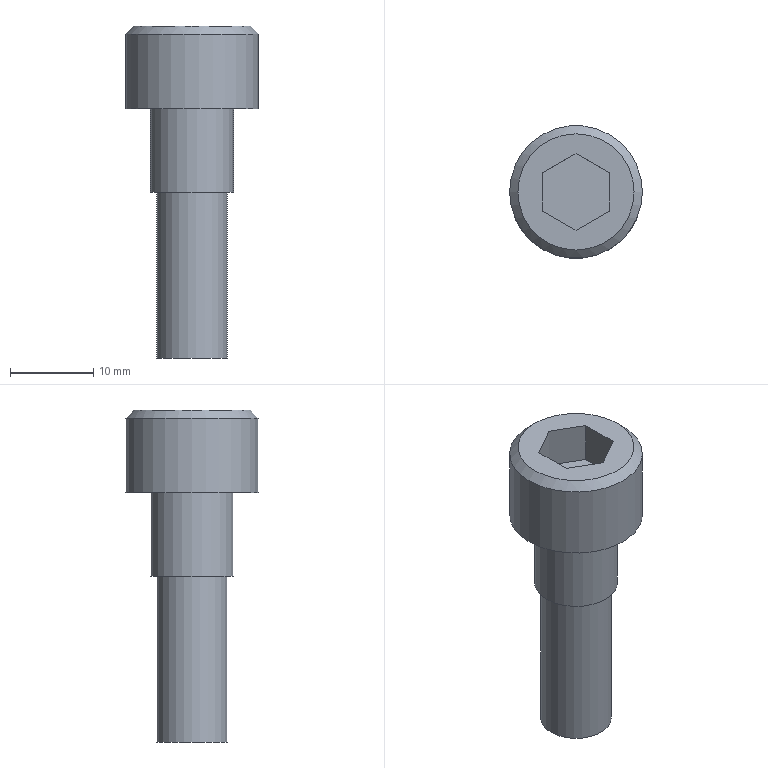Part | STEP file | M3-10_id214_x_t | 1 solid | 15 faces | box 16 x 16 x 40 mm | volume 3630 mm3 | plane 11 | cylinder 3 | cone 1 | commonest cylinder face diameters 8.5 x1 10 x1 16 x1
STEP:
#1=CARTESIAN_POINT('',(140.25,-71.5,-57.));
#2=VERTEX_POINT('',#1);
#3=CARTESIAN_POINT('',(136.,-71.5,-57.));
#4=DIRECTION('',(0.,0.,-1.));
#5=DIRECTION('',(1.,0.,0.));
#6=AXIS2_PLACEMENT_3D('',#3,#4,#5);
#7=CIRCLE('',#6,4.25);
#8=EDGE_CURVE('',#2,#2,#7,.T.);
#9=ORIENTED_EDGE('',*,*,#8,.F.);
#10=EDGE_LOOP('',(#9));
#11=FACE_BOUND('',#10,.T.);
#12=CARTESIAN_POINT('',(131.,-71.5,-57.));
#13=VERTEX_POINT('',#12);
#14=CARTESIAN_POINT('',(136.,-71.5,-57.));
#15=DIRECTION('',(0.,0.,1.));
#16=DIRECTION('',(-1.,0.,0.));
#17=AXIS2_PLACEMENT_3D('',#14,#15,#16);
#18=CIRCLE('',#17,5.);
#19=EDGE_CURVE('',#13,#13,#18,.T.);
#20=ORIENTED_EDGE('',*,*,#19,.F.);
#21=EDGE_LOOP('',(#20));
#22=FACE_BOUND('',#21,.T.);
#23=CARTESIAN_POINT('',(136.,-71.5,-57.));
#24=DIRECTION('',(0.,0.,-1.));
#25=DIRECTION('',(1.,0.,0.));
#26=AXIS2_PLACEMENT_3D('',#23,#24,#25);
#27=PLANE('',#26);
#28=ADVANCED_FACE('',(#11,#22),#27,.T.);
#29=CARTESIAN_POINT('',(141.,-71.5,-47.));
#30=VERTEX_POINT('',#29);
#31=CARTESIAN_POINT('',(136.,-71.5,-47.));
#32=DIRECTION('',(0.,0.,1.));
#33=DIRECTION('',(1.,0.,0.));
#34=AXIS2_PLACEMENT_3D('',#31,#32,#33);
#35=CIRCLE('',#34,5.);
#36=EDGE_CURVE('',#30,#30,#35,.T.);
#37=ORIENTED_EDGE('',*,*,#36,.F.);
#38=EDGE_LOOP('',(#37));
#39=FACE_BOUND('',#38,.T.);
#40=ORIENTED_EDGE('',*,*,#19,.T.);
#41=EDGE_LOOP('',(#40));
#42=FACE_BOUND('',#41,.T.);
#43=CARTESIAN_POINT('',(136.,-71.5,-57.));
#44=DIRECTION('',(0.,0.,1.));
#45=DIRECTION('',(-1.,0.,0.));
#46=AXIS2_PLACEMENT_3D('',#43,#44,#45);
#47=CYLINDRICAL_SURFACE('',#46,5.);
#48=ADVANCED_FACE('',(#39,#42),#47,.T.);
#49=CARTESIAN_POINT('',(131.75,-71.5,-77.));
#50=VERTEX_POINT('',#49);
#51=CARTESIAN_POINT('',(136.,-71.5,-77.));
#52=DIRECTION('',(0.,0.,1.));
#53=DIRECTION('',(-1.,0.,0.));
#54=AXIS2_PLACEMENT_3D('',#51,#52,#53);
#55=CIRCLE('',#54,4.25);
#56=EDGE_CURVE('',#50,#50,#55,.T.);
#57=ORIENTED_EDGE('',*,*,#56,.F.);
#58=EDGE_LOOP('',(#57));
#59=FACE_OUTER_BOUND('',#58,.T.);
#60=CARTESIAN_POINT('',(136.,-71.5,-77.));
#61=DIRECTION('',(0.,0.,-1.));
#62=DIRECTION('',(1.,0.,0.));
#63=AXIS2_PLACEMENT_3D('',#60,#61,#62);
#64=PLANE('',#63);
#65=ADVANCED_FACE('',(#59),#64,.T.);
#66=ORIENTED_EDGE('',*,*,#56,.T.);
#67=EDGE_LOOP('',(#66));
#68=FACE_BOUND('',#67,.T.);
#69=ORIENTED_EDGE('',*,*,#8,.T.);
#70=EDGE_LOOP('',(#69));
#71=FACE_BOUND('',#70,.T.);
#72=CARTESIAN_POINT('',(136.,-71.5,-57.));
#73=DIRECTION('',(0.,0.,-1.));
#74=DIRECTION('',(-1.,0.,0.));
#75=AXIS2_PLACEMENT_3D('',#72,#73,#74);
#76=CYLINDRICAL_SURFACE('',#75,4.25);
#77=ADVANCED_FACE('',(#68,#71),#76,.T.);
#78=CARTESIAN_POINT('',(140.,-73.809,-37.));
#79=VERTEX_POINT('',#78);
#80=CARTESIAN_POINT('',(140.,-69.191,-37.));
#81=VERTEX_POINT('',#80);
#82=CARTESIAN_POINT('',(140.,-73.809,-37.));
#83=DIRECTION('',(0.,1.,0.));
#84=VECTOR('',#83,1.);
#85=LINE('',#82,#84);
#86=EDGE_CURVE('',#79,#81,#85,.T.);
#87=ORIENTED_EDGE('',*,*,#86,.F.);
#88=CARTESIAN_POINT('',(136.,-76.119,-37.));
#89=VERTEX_POINT('',#88);
#90=CARTESIAN_POINT('',(136.,-76.119,-37.));
#91=DIRECTION('',(0.866,0.5,0.));
#92=VECTOR('',#91,1.);
#93=LINE('',#90,#92);
#94=EDGE_CURVE('',#89,#79,#93,.T.);
#95=ORIENTED_EDGE('',*,*,#94,.F.);
#96=CARTESIAN_POINT('',(132.,-73.809,-37.));
#97=VERTEX_POINT('',#96);
#98=CARTESIAN_POINT('',(132.,-73.809,-37.));
#99=DIRECTION('',(0.866,-0.5,0.));
#100=VECTOR('',#99,1.);
#101=LINE('',#98,#100);
#102=EDGE_CURVE('',#97,#89,#101,.T.);
#103=ORIENTED_EDGE('',*,*,#102,.F.);
#104=CARTESIAN_POINT('',(132.,-69.191,-37.));
#105=VERTEX_POINT('',#104);
#106=CARTESIAN_POINT('',(132.,-69.191,-37.));
#107=DIRECTION('',(0.,-1.,0.));
#108=VECTOR('',#107,1.);
#109=LINE('',#106,#108);
#110=EDGE_CURVE('',#105,#97,#109,.T.);
#111=ORIENTED_EDGE('',*,*,#110,.F.);
#112=CARTESIAN_POINT('',(136.,-66.881,-37.));
#113=VERTEX_POINT('',#112);
#114=CARTESIAN_POINT('',(136.,-66.881,-37.));
#115=DIRECTION('',(-0.866,-0.5,0.));
#116=VECTOR('',#115,1.);
#117=LINE('',#114,#116);
#118=EDGE_CURVE('',#113,#105,#117,.T.);
#119=ORIENTED_EDGE('',*,*,#118,.F.);
#120=CARTESIAN_POINT('',(140.,-69.191,-37.));
#121=DIRECTION('',(-0.866,0.5,0.));
#122=VECTOR('',#121,1.);
#123=LINE('',#120,#122);
#124=EDGE_CURVE('',#81,#113,#123,.T.);
#125=ORIENTED_EDGE('',*,*,#124,.F.);
#126=EDGE_LOOP('',(#87,#95,#103,#111,#119,#125));
#127=FACE_BOUND('',#126,.T.);
#128=CARTESIAN_POINT('',(129.,-71.5,-37.));
#129=VERTEX_POINT('',#128);
#130=CARTESIAN_POINT('',(136.,-71.5,-37.));
#131=DIRECTION('',(0.,0.,1.));
#132=DIRECTION('',(-1.,0.,0.));
#133=AXIS2_PLACEMENT_3D('',#130,#131,#132);
#134=CIRCLE('',#133,7.);
#135=EDGE_CURVE('',#129,#129,#134,.T.);
#136=ORIENTED_EDGE('',*,*,#135,.T.);
#137=EDGE_LOOP('',(#136));
#138=FACE_BOUND('',#137,.T.);
#139=CARTESIAN_POINT('',(136.,-71.5,-37.));
#140=DIRECTION('',(0.,0.,1.));
#141=DIRECTION('',(-1.,0.,0.));
#142=AXIS2_PLACEMENT_3D('',#139,#140,#141);
#143=PLANE('',#142);
#144=ADVANCED_FACE('',(#127,#138),#143,.T.);
#145=ORIENTED_EDGE('',*,*,#36,.T.);
#146=EDGE_LOOP('',(#145));
#147=FACE_BOUND('',#146,.T.);
#148=CARTESIAN_POINT('',(128.,-71.5,-47.));
#149=VERTEX_POINT('',#148);
#150=CARTESIAN_POINT('',(136.,-71.5,-47.));
#151=DIRECTION('',(0.,0.,1.));
#152=DIRECTION('',(-1.,0.,0.));
#153=AXIS2_PLACEMENT_3D('',#150,#151,#152);
#154=CIRCLE('',#153,8.);
#155=EDGE_CURVE('',#149,#149,#154,.T.);
#156=ORIENTED_EDGE('',*,*,#155,.F.);
#157=EDGE_LOOP('',(#156));
#158=FACE_BOUND('',#157,.T.);
#159=CARTESIAN_POINT('',(136.,-71.5,-47.));
#160=DIRECTION('',(0.,0.,-1.));
#161=DIRECTION('',(1.,0.,0.));
#162=AXIS2_PLACEMENT_3D('',#159,#160,#161);
#163=PLANE('',#162);
#164=ADVANCED_FACE('',(#147,#158),#163,.T.);
#165=CARTESIAN_POINT('',(128.,-71.5,-38.));
#166=VERTEX_POINT('',#165);
#167=CARTESIAN_POINT('',(136.,-71.5,-38.));
#168=DIRECTION('',(0.,0.,-1.));
#169=DIRECTION('',(-1.,0.,0.));
#170=AXIS2_PLACEMENT_3D('',#167,#168,#169);
#171=CIRCLE('',#170,8.);
#172=EDGE_CURVE('',#166,#166,#171,.T.);
#173=ORIENTED_EDGE('',*,*,#172,.T.);
#174=EDGE_LOOP('',(#173));
#175=FACE_BOUND('',#174,.T.);
#176=ORIENTED_EDGE('',*,*,#155,.T.);
#177=EDGE_LOOP('',(#176));
#178=FACE_BOUND('',#177,.T.);
#179=CARTESIAN_POINT('',(136.,-71.5,-47.));
#180=DIRECTION('',(0.,0.,1.));
#181=DIRECTION('',(-1.,0.,0.));
#182=AXIS2_PLACEMENT_3D('',#179,#180,#181);
#183=CYLINDRICAL_SURFACE('',#182,8.);
#184=ADVANCED_FACE('',(#175,#178),#183,.T.);
#185=ORIENTED_EDGE('',*,*,#135,.F.);
#186=EDGE_LOOP('',(#185));
#187=FACE_BOUND('',#186,.T.);
#188=ORIENTED_EDGE('',*,*,#172,.F.);
#189=EDGE_LOOP('',(#188));
#190=FACE_BOUND('',#189,.T.);
#191=CARTESIAN_POINT('',(136.,-71.5,-38.));
#192=DIRECTION('',(0.,0.,-1.));
#193=DIRECTION('',(1.,0.,0.));
#194=AXIS2_PLACEMENT_3D('',#191,#192,#193);
#195=CONICAL_SURFACE('',#194,8.,45.);
#196=ADVANCED_FACE('',(#187,#190),#195,.T.);
#197=ORIENTED_EDGE('',*,*,#86,.T.);
#198=CARTESIAN_POINT('',(140.,-69.191,-42.));
#199=VERTEX_POINT('',#198);
#200=CARTESIAN_POINT('',(140.,-69.191,-42.));
#201=DIRECTION('',(0.,0.,-1.));
#202=VECTOR('',#201,1.);
#203=LINE('',#200,#202);
#204=EDGE_CURVE('',#81,#199,#203,.T.);
#205=ORIENTED_EDGE('',*,*,#204,.T.);
#206=CARTESIAN_POINT('',(140.,-73.809,-42.));
#207=VERTEX_POINT('',#206);
#208=CARTESIAN_POINT('',(140.,-73.809,-42.));
#209=DIRECTION('',(0.,-1.,0.));
#210=VECTOR('',#209,1.);
#211=LINE('',#208,#210);
#212=EDGE_CURVE('',#199,#207,#211,.T.);
#213=ORIENTED_EDGE('',*,*,#212,.T.);
#214=CARTESIAN_POINT('',(140.,-73.809,-42.));
#215=DIRECTION('',(0.,0.,-1.));
#216=VECTOR('',#215,1.);
#217=LINE('',#214,#216);
#218=EDGE_CURVE('',#79,#207,#217,.T.);
#219=ORIENTED_EDGE('',*,*,#218,.F.);
#220=EDGE_LOOP('',(#197,#205,#213,#219));
#221=FACE_OUTER_BOUND('',#220,.T.);
#222=CARTESIAN_POINT('',(140.,-73.809,-42.));
#223=DIRECTION('',(1.,0.,0.));
#224=DIRECTION('',(0.,1.,0.));
#225=AXIS2_PLACEMENT_3D('',#222,#223,#224);
#226=PLANE('',#225);
#227=ADVANCED_FACE('',(#221),#226,.F.);
#228=ORIENTED_EDGE('',*,*,#124,.T.);
#229=CARTESIAN_POINT('',(136.,-66.881,-42.));
#230=VERTEX_POINT('',#229);
#231=CARTESIAN_POINT('',(136.,-66.881,-42.));
#232=DIRECTION('',(0.,0.,-1.));
#233=VECTOR('',#232,1.);
#234=LINE('',#231,#233);
#235=EDGE_CURVE('',#113,#230,#234,.T.);
#236=ORIENTED_EDGE('',*,*,#235,.T.);
#237=CARTESIAN_POINT('',(140.,-69.191,-42.));
#238=DIRECTION('',(0.866,-0.5,0.));
#239=VECTOR('',#238,1.);
#240=LINE('',#237,#239);
#241=EDGE_CURVE('',#230,#199,#240,.T.);
#242=ORIENTED_EDGE('',*,*,#241,.T.);
#243=ORIENTED_EDGE('',*,*,#204,.F.);
#244=EDGE_LOOP('',(#228,#236,#242,#243));
#245=FACE_OUTER_BOUND('',#244,.T.);
#246=CARTESIAN_POINT('',(140.,-69.191,-42.));
#247=DIRECTION('',(0.5,0.866,0.));
#248=DIRECTION('',(-0.866,0.5,0.));
#249=AXIS2_PLACEMENT_3D('',#246,#247,#248);
#250=PLANE('',#249);
#251=ADVANCED_FACE('',(#245),#250,.F.);
#252=ORIENTED_EDGE('',*,*,#118,.T.);
#253=CARTESIAN_POINT('',(132.,-69.191,-42.));
#254=VERTEX_POINT('',#253);
#255=CARTESIAN_POINT('',(132.,-69.191,-42.));
#256=DIRECTION('',(0.,0.,-1.));
#257=VECTOR('',#256,1.);
#258=LINE('',#255,#257);
#259=EDGE_CURVE('',#105,#254,#258,.T.);
#260=ORIENTED_EDGE('',*,*,#259,.T.);
#261=CARTESIAN_POINT('',(136.,-66.881,-42.));
#262=DIRECTION('',(0.866,0.5,0.));
#263=VECTOR('',#262,1.);
#264=LINE('',#261,#263);
#265=EDGE_CURVE('',#254,#230,#264,.T.);
#266=ORIENTED_EDGE('',*,*,#265,.T.);
#267=ORIENTED_EDGE('',*,*,#235,.F.);
#268=EDGE_LOOP('',(#252,#260,#266,#267));
#269=FACE_OUTER_BOUND('',#268,.T.);
#270=CARTESIAN_POINT('',(136.,-66.881,-42.));
#271=DIRECTION('',(-0.5,0.866,0.));
#272=DIRECTION('',(-0.866,-0.5,0.));
#273=AXIS2_PLACEMENT_3D('',#270,#271,#272);
#274=PLANE('',#273);
#275=ADVANCED_FACE('',(#269),#274,.F.);
#276=ORIENTED_EDGE('',*,*,#110,.T.);
#277=CARTESIAN_POINT('',(132.,-73.809,-42.));
#278=VERTEX_POINT('',#277);
#279=CARTESIAN_POINT('',(132.,-73.809,-42.));
#280=DIRECTION('',(0.,0.,-1.));
#281=VECTOR('',#280,1.);
#282=LINE('',#279,#281);
#283=EDGE_CURVE('',#97,#278,#282,.T.);
#284=ORIENTED_EDGE('',*,*,#283,.T.);
#285=CARTESIAN_POINT('',(132.,-69.191,-42.));
#286=DIRECTION('',(0.,1.,0.));
#287=VECTOR('',#286,1.);
#288=LINE('',#285,#287);
#289=EDGE_CURVE('',#278,#254,#288,.T.);
#290=ORIENTED_EDGE('',*,*,#289,.T.);
#291=ORIENTED_EDGE('',*,*,#259,.F.);
#292=EDGE_LOOP('',(#276,#284,#290,#291));
#293=FACE_OUTER_BOUND('',#292,.T.);
#294=CARTESIAN_POINT('',(132.,-69.191,-42.));
#295=DIRECTION('',(-1.,0.,0.));
#296=DIRECTION('',(0.,-1.,0.));
#297=AXIS2_PLACEMENT_3D('',#294,#295,#296);
#298=PLANE('',#297);
#299=ADVANCED_FACE('',(#293),#298,.F.);
#300=ORIENTED_EDGE('',*,*,#102,.T.);
#301=CARTESIAN_POINT('',(136.,-76.119,-42.));
#302=VERTEX_POINT('',#301);
#303=CARTESIAN_POINT('',(136.,-76.119,-42.));
#304=DIRECTION('',(0.,0.,-1.));
#305=VECTOR('',#304,1.);
#306=LINE('',#303,#305);
#307=EDGE_CURVE('',#89,#302,#306,.T.);
#308=ORIENTED_EDGE('',*,*,#307,.T.);
#309=CARTESIAN_POINT('',(132.,-73.809,-42.));
#310=DIRECTION('',(-0.866,0.5,0.));
#311=VECTOR('',#310,1.);
#312=LINE('',#309,#311);
#313=EDGE_CURVE('',#302,#278,#312,.T.);
#314=ORIENTED_EDGE('',*,*,#313,.T.);
#315=ORIENTED_EDGE('',*,*,#283,.F.);
#316=EDGE_LOOP('',(#300,#308,#314,#315));
#317=FACE_OUTER_BOUND('',#316,.T.);
#318=CARTESIAN_POINT('',(132.,-73.809,-42.));
#319=DIRECTION('',(-0.5,-0.866,0.));
#320=DIRECTION('',(0.866,-0.5,0.));
#321=AXIS2_PLACEMENT_3D('',#318,#319,#320);
#322=PLANE('',#321);
#323=ADVANCED_FACE('',(#317),#322,.F.);
#324=ORIENTED_EDGE('',*,*,#94,.T.);
#325=ORIENTED_EDGE('',*,*,#218,.T.);
#326=CARTESIAN_POINT('',(136.,-76.119,-42.));
#327=DIRECTION('',(-0.866,-0.5,0.));
#328=VECTOR('',#327,1.);
#329=LINE('',#326,#328);
#330=EDGE_CURVE('',#207,#302,#329,.T.);
#331=ORIENTED_EDGE('',*,*,#330,.T.);
#332=ORIENTED_EDGE('',*,*,#307,.F.);
#333=EDGE_LOOP('',(#324,#325,#331,#332));
#334=FACE_OUTER_BOUND('',#333,.T.);
#335=CARTESIAN_POINT('',(136.,-76.119,-42.));
#336=DIRECTION('',(0.5,-0.866,0.));
#337=DIRECTION('',(0.866,0.5,0.));
#338=AXIS2_PLACEMENT_3D('',#335,#336,#337);
#339=PLANE('',#338);
#340=ADVANCED_FACE('',(#334),#339,.F.);
#341=ORIENTED_EDGE('',*,*,#212,.F.);
#342=ORIENTED_EDGE('',*,*,#241,.F.);
#343=ORIENTED_EDGE('',*,*,#265,.F.);
#344=ORIENTED_EDGE('',*,*,#289,.F.);
#345=ORIENTED_EDGE('',*,*,#313,.F.);
#346=ORIENTED_EDGE('',*,*,#330,.F.);
#347=EDGE_LOOP('',(#341,#342,#343,#344,#345,#346));
#348=FACE_OUTER_BOUND('',#347,.T.);
#349=CARTESIAN_POINT('',(136.,-71.5,-42.));
#350=DIRECTION('',(0.,0.,1.));
#351=DIRECTION('',(-1.,0.,0.));
#352=AXIS2_PLACEMENT_3D('',#349,#350,#351);
#353=PLANE('',#352);
#354=ADVANCED_FACE('',(#348),#353,.T.);
#355=CLOSED_SHELL('',(#28,#48,#65,#77,#144,#164,#184,#196,#227,#251,#275,#299,#323,#340,#354));
#356=MANIFOLD_SOLID_BREP('',#355);
#357=(LENGTH_UNIT()NAMED_UNIT(*)SI_UNIT(.MILLI.,.METRE.));
#358=UNCERTAINTY_MEASURE_WITH_UNIT(LENGTH_MEASURE(0.00002),#357,'','');
#359=(NAMED_UNIT(*)PLANE_ANGLE_UNIT()SI_UNIT($,.RADIAN.));
#360=PLANE_ANGLE_MEASURE_WITH_UNIT(PLANE_ANGLE_MEASURE(0.01745),#359);
#361=DIMENSIONAL_EXPONENTS(0.,0.,0.,0.,0.,0.,0.);
#362=(CONVERSION_BASED_UNIT('DEGREE',#360)NAMED_UNIT(#361)PLANE_ANGLE_UNIT());
#363=(NAMED_UNIT(*)SI_UNIT($,.STERADIAN.)SOLID_ANGLE_UNIT());
#364=(GEOMETRIC_REPRESENTATION_CONTEXT(3)GLOBAL_UNCERTAINTY_ASSIGNED_CONTEXT((#358))GLOBAL_UNIT_ASSIGNED_CONTEXT((#357,#362,#363))REPRESENTATION_CONTEXT('',''));
#365=ADVANCED_BREP_SHAPE_REPRESENTATION('',(#356),#364);